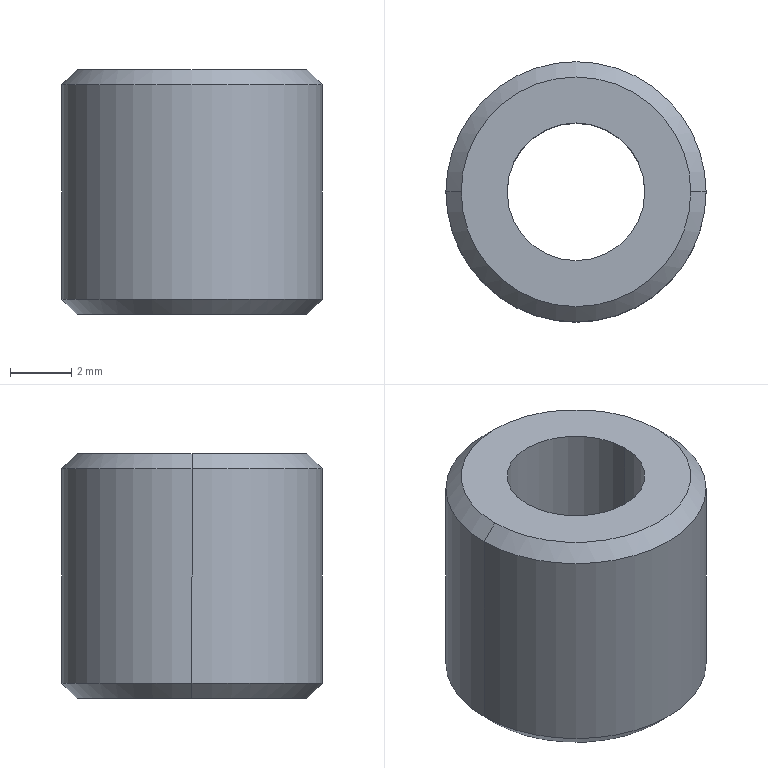Part | STEP file | CHAIN-01_1_02LT_1-2 | 1 solid | 10 faces | box 8.5 x 8.5 x 8 mm | volume 320.312 mm3 | cylinder 4 | cone 4 | plane 2 | commonest cylinder face diameters 4.5 x2 8.5 x2
STEP:
#1=CARTESIAN_POINT('',(4.25,0.,-3.5));
#2=VERTEX_POINT('',#1);
#3=CARTESIAN_POINT('',(-4.25,0.,-3.5));
#4=VERTEX_POINT('',#3);
#5=CARTESIAN_POINT('',(0.,0.,-3.5));
#6=DIRECTION('',(0.,0.,1.));
#7=DIRECTION('',(1.,0.,0.));
#8=AXIS2_PLACEMENT_3D('',#5,#6,#7);
#9=CIRCLE('',#8,4.25);
#10=EDGE_CURVE('',#2,#4,#9,.T.);
#11=ORIENTED_EDGE('',*,*,#10,.T.);
#12=CARTESIAN_POINT('',(-4.25,0.,3.5));
#13=VERTEX_POINT('',#12);
#14=CARTESIAN_POINT('',(-4.25,0.,-4.));
#15=DIRECTION('',(0.,0.,1.));
#16=VECTOR('',#15,1000.);
#17=LINE('',#14,#16);
#18=EDGE_CURVE('',#4,#13,#17,.T.);
#19=ORIENTED_EDGE('',*,*,#18,.T.);
#20=CARTESIAN_POINT('',(4.25,0.,3.5));
#21=VERTEX_POINT('',#20);
#22=CARTESIAN_POINT('',(0.,0.,3.5));
#23=DIRECTION('',(0.,0.,-1.));
#24=DIRECTION('',(1.,0.,0.));
#25=AXIS2_PLACEMENT_3D('',#22,#23,#24);
#26=CIRCLE('',#25,4.25);
#27=EDGE_CURVE('',#13,#21,#26,.T.);
#28=ORIENTED_EDGE('',*,*,#27,.T.);
#29=CARTESIAN_POINT('',(4.25,0.,-4.));
#30=DIRECTION('',(0.,0.,1.));
#31=VECTOR('',#30,1000.);
#32=LINE('',#29,#31);
#33=EDGE_CURVE('',#2,#21,#32,.T.);
#34=ORIENTED_EDGE('',*,*,#33,.F.);
#35=EDGE_LOOP('',(#11,#19,#28,#34));
#36=FACE_OUTER_BOUND('',#35,.T.);
#37=CARTESIAN_POINT('',(0.,0.,-4.));
#38=DIRECTION('',(0.,0.,1.));
#39=DIRECTION('',(1.,0.,0.));
#40=AXIS2_PLACEMENT_3D('',#37,#38,#39);
#41=CYLINDRICAL_SURFACE('',#40,4.25);
#42=ADVANCED_FACE('',(#36),#41,.T.);
#43=CARTESIAN_POINT('',(3.75,0.,-4.));
#44=VERTEX_POINT('',#43);
#45=CARTESIAN_POINT('',(-3.75,0.,-4.));
#46=VERTEX_POINT('',#45);
#47=CARTESIAN_POINT('',(0.,0.,-4.));
#48=DIRECTION('',(0.,0.,1.));
#49=DIRECTION('',(1.,0.,0.));
#50=AXIS2_PLACEMENT_3D('',#47,#48,#49);
#51=CIRCLE('',#50,3.75);
#52=EDGE_CURVE('',#44,#46,#51,.T.);
#53=ORIENTED_EDGE('',*,*,#52,.T.);
#54=CARTESIAN_POINT('',(-4.25,0.,-3.5));
#55=DIRECTION('',(-0.7071,0.,0.7071));
#56=VECTOR('',#55,1000.);
#57=LINE('',#54,#56);
#58=EDGE_CURVE('',#46,#4,#57,.T.);
#59=ORIENTED_EDGE('',*,*,#58,.T.);
#60=ORIENTED_EDGE('',*,*,#10,.F.);
#61=CARTESIAN_POINT('',(4.25,0.,-3.5));
#62=DIRECTION('',(0.7071,0.,0.7071));
#63=VECTOR('',#62,1000.);
#64=LINE('',#61,#63);
#65=EDGE_CURVE('',#44,#2,#64,.T.);
#66=ORIENTED_EDGE('',*,*,#65,.F.);
#67=EDGE_LOOP('',(#53,#59,#60,#66));
#68=FACE_OUTER_BOUND('',#67,.T.);
#69=CARTESIAN_POINT('',(0.,0.,-3.5));
#70=DIRECTION('',(0.,0.,1.));
#71=DIRECTION('',(1.,0.,0.));
#72=AXIS2_PLACEMENT_3D('',#69,#70,#71);
#73=CONICAL_SURFACE('',#72,4.25,0.7854);
#74=ADVANCED_FACE('',(#68),#73,.T.);
#75=CARTESIAN_POINT('',(-3.75,0.,4.));
#76=VERTEX_POINT('',#75);
#77=CARTESIAN_POINT('',(3.75,0.,4.));
#78=VERTEX_POINT('',#77);
#79=CARTESIAN_POINT('',(0.,0.,4.));
#80=DIRECTION('',(0.,0.,-1.));
#81=DIRECTION('',(-1.,0.,0.));
#82=AXIS2_PLACEMENT_3D('',#79,#80,#81);
#83=CIRCLE('',#82,3.75);
#84=EDGE_CURVE('',#76,#78,#83,.T.);
#85=ORIENTED_EDGE('',*,*,#84,.T.);
#86=CARTESIAN_POINT('',(4.25,0.,3.5));
#87=DIRECTION('',(0.7071,0.,-0.7071));
#88=VECTOR('',#87,1000.);
#89=LINE('',#86,#88);
#90=EDGE_CURVE('',#78,#21,#89,.T.);
#91=ORIENTED_EDGE('',*,*,#90,.T.);
#92=ORIENTED_EDGE('',*,*,#27,.F.);
#93=CARTESIAN_POINT('',(-4.25,0.,3.5));
#94=DIRECTION('',(-0.7071,0.,-0.7071));
#95=VECTOR('',#94,1000.);
#96=LINE('',#93,#95);
#97=EDGE_CURVE('',#76,#13,#96,.T.);
#98=ORIENTED_EDGE('',*,*,#97,.F.);
#99=EDGE_LOOP('',(#85,#91,#92,#98));
#100=FACE_OUTER_BOUND('',#99,.T.);
#101=CARTESIAN_POINT('',(0.,0.,3.5));
#102=DIRECTION('',(0.,0.,-1.));
#103=DIRECTION('',(-1.,0.,0.));
#104=AXIS2_PLACEMENT_3D('',#101,#102,#103);
#105=CONICAL_SURFACE('',#104,4.25,0.7854);
#106=ADVANCED_FACE('',(#100),#105,.T.);
#107=CARTESIAN_POINT('',(2.25,0.,-4.));
#108=VERTEX_POINT('',#107);
#109=CARTESIAN_POINT('',(-2.25,0.,-4.));
#110=VERTEX_POINT('',#109);
#111=CARTESIAN_POINT('',(0.,0.,-4.));
#112=DIRECTION('',(0.,0.,-1.));
#113=DIRECTION('',(1.,0.,0.));
#114=AXIS2_PLACEMENT_3D('',#111,#112,#113);
#115=CIRCLE('',#114,2.25);
#116=EDGE_CURVE('',#108,#110,#115,.T.);
#117=ORIENTED_EDGE('',*,*,#116,.T.);
#118=CARTESIAN_POINT('',(-2.25,0.,4.));
#119=VERTEX_POINT('',#118);
#120=CARTESIAN_POINT('',(-2.25,0.,-4.));
#121=DIRECTION('',(0.,0.,1.));
#122=VECTOR('',#121,1000.);
#123=LINE('',#120,#122);
#124=EDGE_CURVE('',#110,#119,#123,.T.);
#125=ORIENTED_EDGE('',*,*,#124,.T.);
#126=CARTESIAN_POINT('',(2.25,0.,4.));
#127=VERTEX_POINT('',#126);
#128=CARTESIAN_POINT('',(0.,0.,4.));
#129=DIRECTION('',(0.,0.,-1.));
#130=DIRECTION('',(1.,0.,0.));
#131=AXIS2_PLACEMENT_3D('',#128,#129,#130);
#132=CIRCLE('',#131,2.25);
#133=EDGE_CURVE('',#127,#119,#132,.T.);
#134=ORIENTED_EDGE('',*,*,#133,.F.);
#135=CARTESIAN_POINT('',(2.25,0.,-4.));
#136=DIRECTION('',(0.,0.,1.));
#137=VECTOR('',#136,1000.);
#138=LINE('',#135,#137);
#139=EDGE_CURVE('',#108,#127,#138,.T.);
#140=ORIENTED_EDGE('',*,*,#139,.F.);
#141=EDGE_LOOP('',(#117,#125,#134,#140));
#142=FACE_OUTER_BOUND('',#141,.T.);
#143=CARTESIAN_POINT('',(0.,0.,-4.));
#144=DIRECTION('',(0.,0.,1.));
#145=DIRECTION('',(1.,0.,0.));
#146=AXIS2_PLACEMENT_3D('',#143,#144,#145);
#147=CYLINDRICAL_SURFACE('',#146,2.25);
#148=ADVANCED_FACE('',(#142),#147,.F.);
#149=ORIENTED_EDGE('',*,*,#18,.F.);
#150=CARTESIAN_POINT('',(0.,0.,-3.5));
#151=DIRECTION('',(0.,0.,1.));
#152=DIRECTION('',(1.,0.,0.));
#153=AXIS2_PLACEMENT_3D('',#150,#151,#152);
#154=CIRCLE('',#153,4.25);
#155=EDGE_CURVE('',#4,#2,#154,.T.);
#156=ORIENTED_EDGE('',*,*,#155,.T.);
#157=ORIENTED_EDGE('',*,*,#33,.T.);
#158=CARTESIAN_POINT('',(0.,0.,3.5));
#159=DIRECTION('',(0.,0.,-1.));
#160=DIRECTION('',(1.,0.,0.));
#161=AXIS2_PLACEMENT_3D('',#158,#159,#160);
#162=CIRCLE('',#161,4.25);
#163=EDGE_CURVE('',#21,#13,#162,.T.);
#164=ORIENTED_EDGE('',*,*,#163,.T.);
#165=EDGE_LOOP('',(#149,#156,#157,#164));
#166=FACE_OUTER_BOUND('',#165,.T.);
#167=CARTESIAN_POINT('',(0.,0.,-4.));
#168=DIRECTION('',(0.,0.,1.));
#169=DIRECTION('',(1.,0.,0.));
#170=AXIS2_PLACEMENT_3D('',#167,#168,#169);
#171=CYLINDRICAL_SURFACE('',#170,4.25);
#172=ADVANCED_FACE('',(#166),#171,.T.);
#173=ORIENTED_EDGE('',*,*,#58,.F.);
#174=CARTESIAN_POINT('',(0.,0.,-4.));
#175=DIRECTION('',(0.,0.,1.));
#176=DIRECTION('',(1.,0.,0.));
#177=AXIS2_PLACEMENT_3D('',#174,#175,#176);
#178=CIRCLE('',#177,3.75);
#179=EDGE_CURVE('',#46,#44,#178,.T.);
#180=ORIENTED_EDGE('',*,*,#179,.T.);
#181=ORIENTED_EDGE('',*,*,#65,.T.);
#182=ORIENTED_EDGE('',*,*,#155,.F.);
#183=EDGE_LOOP('',(#173,#180,#181,#182));
#184=FACE_OUTER_BOUND('',#183,.T.);
#185=CARTESIAN_POINT('',(0.,0.,-3.5));
#186=DIRECTION('',(0.,0.,1.));
#187=DIRECTION('',(1.,0.,0.));
#188=AXIS2_PLACEMENT_3D('',#185,#186,#187);
#189=CONICAL_SURFACE('',#188,4.25,0.7854);
#190=ADVANCED_FACE('',(#184),#189,.T.);
#191=ORIENTED_EDGE('',*,*,#90,.F.);
#192=CARTESIAN_POINT('',(0.,0.,4.));
#193=DIRECTION('',(0.,0.,-1.));
#194=DIRECTION('',(-1.,0.,0.));
#195=AXIS2_PLACEMENT_3D('',#192,#193,#194);
#196=CIRCLE('',#195,3.75);
#197=EDGE_CURVE('',#78,#76,#196,.T.);
#198=ORIENTED_EDGE('',*,*,#197,.T.);
#199=ORIENTED_EDGE('',*,*,#97,.T.);
#200=ORIENTED_EDGE('',*,*,#163,.F.);
#201=EDGE_LOOP('',(#191,#198,#199,#200));
#202=FACE_OUTER_BOUND('',#201,.T.);
#203=CARTESIAN_POINT('',(0.,0.,3.5));
#204=DIRECTION('',(0.,0.,-1.));
#205=DIRECTION('',(-1.,0.,0.));
#206=AXIS2_PLACEMENT_3D('',#203,#204,#205);
#207=CONICAL_SURFACE('',#206,4.25,0.7854);
#208=ADVANCED_FACE('',(#202),#207,.T.);
#209=ORIENTED_EDGE('',*,*,#116,.F.);
#210=CARTESIAN_POINT('',(0.,0.,-4.));
#211=DIRECTION('',(0.,0.,-1.));
#212=DIRECTION('',(1.,0.,0.));
#213=AXIS2_PLACEMENT_3D('',#210,#211,#212);
#214=CIRCLE('',#213,2.25);
#215=EDGE_CURVE('',#110,#108,#214,.T.);
#216=ORIENTED_EDGE('',*,*,#215,.F.);
#217=EDGE_LOOP('',(#209,#216));
#218=FACE_BOUND('',#217,.T.);
#219=ORIENTED_EDGE('',*,*,#52,.F.);
#220=ORIENTED_EDGE('',*,*,#179,.F.);
#221=EDGE_LOOP('',(#219,#220));
#222=FACE_OUTER_BOUND('',#221,.T.);
#223=CARTESIAN_POINT('',(0.,0.,-4.));
#224=DIRECTION('',(0.,0.,1.));
#225=DIRECTION('',(1.,0.,0.));
#226=AXIS2_PLACEMENT_3D('',#223,#224,#225);
#227=PLANE('',#226);
#228=ADVANCED_FACE('',(#218,#222),#227,.F.);
#229=ORIENTED_EDGE('',*,*,#133,.T.);
#230=CARTESIAN_POINT('',(0.,0.,4.));
#231=DIRECTION('',(0.,0.,-1.));
#232=DIRECTION('',(1.,0.,0.));
#233=AXIS2_PLACEMENT_3D('',#230,#231,#232);
#234=CIRCLE('',#233,2.25);
#235=EDGE_CURVE('',#119,#127,#234,.T.);
#236=ORIENTED_EDGE('',*,*,#235,.T.);
#237=EDGE_LOOP('',(#229,#236));
#238=FACE_BOUND('',#237,.T.);
#239=ORIENTED_EDGE('',*,*,#84,.F.);
#240=ORIENTED_EDGE('',*,*,#197,.F.);
#241=EDGE_LOOP('',(#239,#240));
#242=FACE_OUTER_BOUND('',#241,.T.);
#243=CARTESIAN_POINT('',(0.,0.,4.));
#244=DIRECTION('',(0.,0.,1.));
#245=DIRECTION('',(1.,0.,0.));
#246=AXIS2_PLACEMENT_3D('',#243,#244,#245);
#247=PLANE('',#246);
#248=ADVANCED_FACE('',(#238,#242),#247,.T.);
#249=ORIENTED_EDGE('',*,*,#124,.F.);
#250=ORIENTED_EDGE('',*,*,#215,.T.);
#251=ORIENTED_EDGE('',*,*,#139,.T.);
#252=ORIENTED_EDGE('',*,*,#235,.F.);
#253=EDGE_LOOP('',(#249,#250,#251,#252));
#254=FACE_OUTER_BOUND('',#253,.T.);
#255=CARTESIAN_POINT('',(0.,0.,-4.));
#256=DIRECTION('',(0.,0.,1.));
#257=DIRECTION('',(1.,0.,0.));
#258=AXIS2_PLACEMENT_3D('',#255,#256,#257);
#259=CYLINDRICAL_SURFACE('',#258,2.25);
#260=ADVANCED_FACE('',(#254),#259,.F.);
#261=CLOSED_SHELL('',(#42,#74,#106,#148,#172,#190,#208,#228,#248,#260));
#262=MANIFOLD_SOLID_BREP('',#261);
#263=CARTESIAN_POINT('',(0.,0.,0.));
#264=DIRECTION('',(0.,0.,1.));
#265=DIRECTION('',(1.,0.,0.));
#266=AXIS2_PLACEMENT_3D('',#263,#264,#265);
#267=(LENGTH_UNIT()NAMED_UNIT(*)SI_UNIT(.MILLI.,.METRE.));
#268=UNCERTAINTY_MEASURE_WITH_UNIT(LENGTH_MEASURE(0.00001),#267,'','');
#269=(NAMED_UNIT(*)PLANE_ANGLE_UNIT()SI_UNIT($,.RADIAN.));
#270=(NAMED_UNIT(*)SI_UNIT($,.STERADIAN.)SOLID_ANGLE_UNIT());
#271=(GEOMETRIC_REPRESENTATION_CONTEXT(3)GLOBAL_UNCERTAINTY_ASSIGNED_CONTEXT((#268))GLOBAL_UNIT_ASSIGNED_CONTEXT((#267,#269,#270))REPRESENTATION_CONTEXT('',''));
#272=ADVANCED_BREP_SHAPE_REPRESENTATION('',(#262,#266),#271);